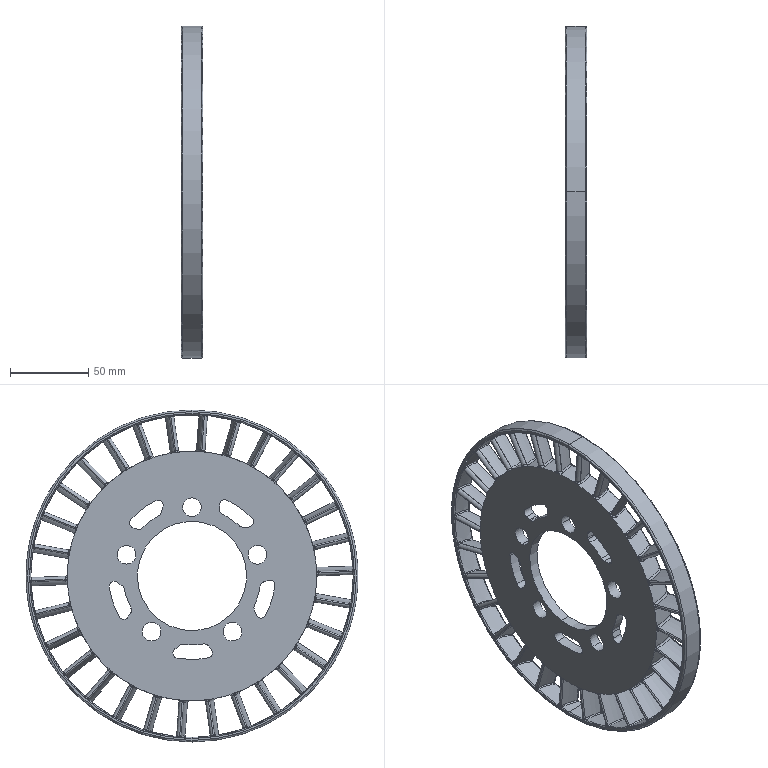Part | STEP file | Completa.sldasm-Part-27_Valor predeterminado | 1 solid | 949 faces | box 14 x 212.474 x 212.474 mm | volume 171916 mm3 | spline 540 | cylinder 321 | torus 73 | plane 15 | commonest cylinder face diameters 1.1 x60 4.4 x60 159.5 x31 206.474 x31 1.32 x30 58.884 x30